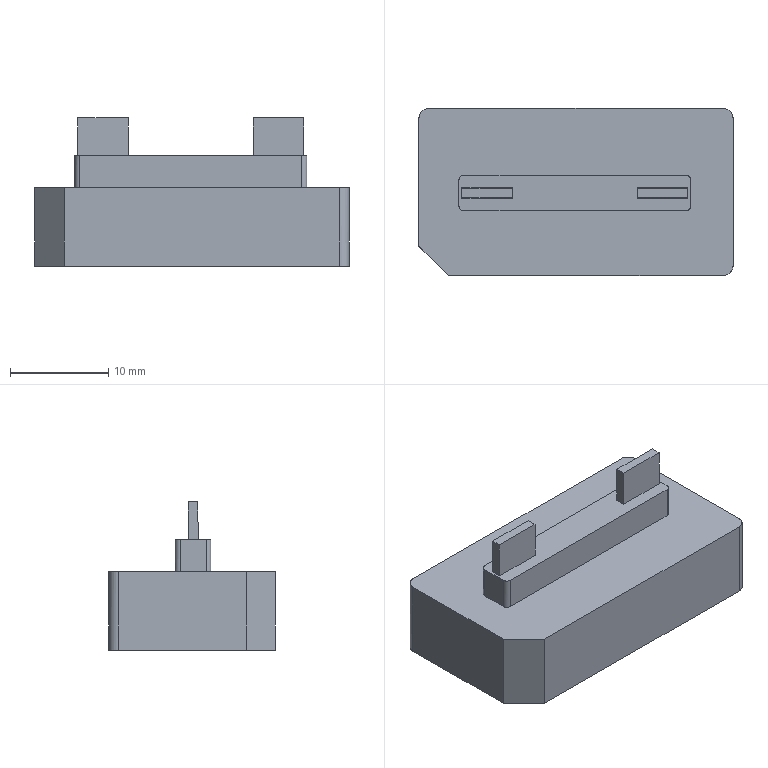NC program | PowerMill | posted by the shop | part box 32 x 17 x 15.109 mm
Lines 1 to 1597 of 56729:
%
G40 G49 G17 G80
( TOOL ID   D10C_1_1 )
( TOOL DIA. 10. TIP RAD 0 LENGTH 70.56 )
( Z = -.071 )
T1 M6
T3
G91 G28 Z0
G0 G90 G54
M08
S8000 M3
G0 X0 Y0 M8
G43 Z10.2 H1
X23.78 Y11.28
Z1.129
G1 Z-.071 F6000
X18.78 F10000
X-18.78
Y5.64
X18.78
Y0
X-18.78
Y-5.64
X18.78
Y-11.28
X-18.78
X-23.78
G0 Z10.2
X-.12 Y0
Z9.879
X24.737 Y5.134
Z.697
G1 Z-.503 F6000
X24.209 F10000
G3 X19.462 Y.387 I0 J-4.748
G1 Y-10.28
G2 X18.462 Y-11.28 I-1. J0
G1 X-18.702
G2 X-19.702 Y-10.28 I0 J1.
G1 Y10.28
G2 X-18.702 Y11.28 I1. J0
G1 X18.462
G2 X19.462 Y10.28 I0 J-1.
G1 Y.387
X16.663
Y-.387
X16.632 Y-1.16
X16.488 Y-1.934
X16.222 Y-2.707
X15.804 Y-3.48
X15.349 Y-4.081
X15.187 Y-4.254
X14.575 Y-4.799
X14.254 Y-5.027
X13.802 Y-5.289
X13.028 Y-5.611
X12.272 Y-5.801
X11.481 Y-5.872
X6.067 Y-5.87
X5.365 Y-5.801
X4.521 Y-5.583
X3.747 Y-5.243
X3.384 Y-5.027
X2.974 Y-4.733
X2.446 Y-4.254
X2.2 Y-3.978
X1.831 Y-3.48
X1.427 Y-2.736
X1.147 Y-1.934
X1.005 Y-1.16
X.979 Y.387
X-1.214
Y-.387
X-1.244 Y-1.16
X-1.389 Y-1.934
X-1.654 Y-2.707
X-2.071 Y-3.48
X-2.44 Y-3.978
X-2.686 Y-4.254
X-3.214 Y-4.733
X-3.623 Y-5.027
X-3.987 Y-5.243
X-4.761 Y-5.583
X-5.605 Y-5.801
X-6.307 Y-5.87
X-11.721 Y-5.872
X-12.495 Y-5.803
X-13.268 Y-5.611
X-14.042 Y-5.289
X-14.493 Y-5.027
X-14.815 Y-4.799
X-15.43 Y-4.254
X-15.589 Y-4.081
X-16.045 Y-3.48
X-16.462 Y-2.707
X-16.73 Y-1.934
X-16.872 Y-1.16
X-16.903 Y-.387
Y.387
X-16.838 Y1.16
X-16.661 Y1.934
X-16.362 Y2.699
X-15.886 Y3.48
X-15.589 Y3.855
X-15.201 Y4.254
X-14.815 Y4.574
X-14.113 Y5.027
X-13.268 Y5.386
X-12.495 Y5.578
X-11.721 Y5.651
X-6.307 Y5.649
X-5.534 Y5.564
X-4.761 Y5.359
X-4.003 Y5.027
X-3.214 Y4.509
X-2.916 Y4.254
X-2.44 Y3.755
X-2.227 Y3.48
X-1.758 Y2.707
X-1.453 Y1.934
X-1.273 Y1.16
X-1.214 Y.387
X.979
X1.036 Y1.16
X1.212 Y1.934
X1.518 Y2.707
X1.987 Y3.48
X2.2 Y3.755
X2.675 Y4.254
X2.974 Y4.509
X3.747 Y5.019
X4.521 Y5.359
X5.294 Y5.564
X6.067 Y5.649
X11.481 Y5.651
X12.255 Y5.578
X13.028 Y5.386
X13.802 Y5.065
X14.575 Y4.574
X14.962 Y4.254
X15.349 Y3.855
X15.651 Y3.48
X16.118 Y2.707
X16.421 Y1.934
X16.602 Y1.16
X16.663 Y.387
X19.462
G0 Z3.315
G1 X24.737 Y5.134
G0 Z.315
G1 Z-.885 F6000
X24.209 F10000
G3 X19.462 Y.387 I0 J-4.748
G1 Y.333
X16.663 Y.387
X16.662 Y.384
X16.663 Y-.387
X16.633 Y-1.137
Y-1.16
X16.49 Y-1.934
X16.224 Y-2.707
X15.807 Y-3.48
X15.349 Y-4.085
X15.193 Y-4.254
X14.575 Y-4.805
X14.259 Y-5.027
X13.802 Y-5.293
X13.028 Y-5.616
X12.29 Y-5.801
X11.481 Y-5.879
X6.067 Y-5.876
X5.343 Y-5.801
X4.521 Y-5.588
X3.747 Y-5.248
X3.374 Y-5.027
X2.974 Y-4.74
X2.44 Y-4.254
X2.2 Y-3.987
X1.826 Y-3.48
X1.427 Y-2.746
X1.142 Y-1.934
X1. Y-1.16
X.971 Y.345
X-1.211 Y.387
X-1.214 Y.211
Y-.387
X-1.237 Y-.971
X-1.24 Y-1.16
X-1.382 Y-1.934
X-1.649 Y-2.707
X-2.066 Y-3.48
X-2.44 Y-3.987
X-2.68 Y-4.254
X-3.214 Y-4.74
X-3.614 Y-5.027
X-3.987 Y-5.248
X-4.761 Y-5.588
X-5.583 Y-5.801
X-6.307 Y-5.876
X-11.721 Y-5.879
X-12.495 Y-5.807
X-13.268 Y-5.616
X-14.042 Y-5.293
X-14.499 Y-5.027
X-14.815 Y-4.805
X-15.434 Y-4.254
X-15.589 Y-4.085
X-16.047 Y-3.48
X-16.464 Y-2.707
X-16.731 Y-1.934
X-16.873 Y-1.16
X-16.874 Y-1.12
X-16.902 Y-.387
Y.384
X-16.903 Y.387
X-16.844 Y1.16
X-16.666 Y1.934
X-16.362 Y2.703
X-15.893 Y3.48
X-15.589 Y3.86
X-15.205 Y4.254
X-14.815 Y4.581
X-14.12 Y5.027
X-13.268 Y5.391
X-12.495 Y5.583
X-11.721 Y5.654
X-6.307 Y5.652
X-5.534 Y5.568
X-4.761 Y5.364
X-3.993 Y5.027
X-3.214 Y4.515
X-2.908 Y4.254
X-2.44 Y3.762
X-2.22 Y3.48
X-1.753 Y2.707
X-1.446 Y1.934
X-1.269 Y1.16
X-1.211 Y.387
X.971 Y.345
Y.387
X1.03 Y1.16
X1.206 Y1.934
X1.513 Y2.707
X1.98 Y3.48
X2.2 Y3.762
X2.668 Y4.254
X2.974 Y4.515
X3.747 Y5.024
X4.521 Y5.364
X5.294 Y5.568
X6.067 Y5.652
X11.481 Y5.654
X12.255 Y5.583
X13.028 Y5.391
X13.802 Y5.069
X14.575 Y4.581
X14.965 Y4.254
X15.349 Y3.86
X15.653 Y3.48
X16.12 Y2.707
X16.426 Y1.934
X16.604 Y1.16
X16.663 Y.387
X19.462 Y.333
Y-10.28
G2 X18.462 Y-11.28 I-1. J0
G1 X-18.702
G2 X-19.702 Y-10.28 I0 J1.
G1 Y10.28
G2 X-18.702 Y11.28 I1. J0
G1 X18.462
G2 X19.462 Y10.28 I0 J-1.
G1 Y.387
G0 Z2.934
G1 X24.737 Y5.134
G0 Z-.066
G1 Z-1.266 F6000
X24.209 F10000
G3 X19.462 Y.387 I0 J-4.748
G1 Y.333
X16.663 Y.387
X16.662 Y.38
Y-.387
X16.634 Y-1.117
X16.633 Y-1.16
X16.492 Y-1.934
X16.225 Y-2.707
X15.81 Y-3.48
X15.349 Y-4.088
X15.197 Y-4.254
X14.575 Y-4.808
X14.264 Y-5.027
X13.802 Y-5.296
X13.028 Y-5.62
X12.309 Y-5.801
X11.481 Y-5.882
X6.067 Y-5.88
X5.321 Y-5.801
X4.521 Y-5.592
X3.747 Y-5.253
X3.366 Y-5.027
X2.974 Y-4.745
X2.433 Y-4.254
X2.2 Y-3.994
X1.82 Y-3.48
X1.427 Y-2.757
X1.138 Y-1.934
X.997 Y-1.16
X.968 Y.345
X-1.207 Y.387
X-1.214 Y.032
Y-.387
X-1.23 Y-.786
X-1.237 Y-1.16
X-1.378 Y-1.934
X-1.645 Y-2.707
X-2.06 Y-3.48
X-2.44 Y-3.994
X-2.673 Y-4.254
X-3.214 Y-4.745
X-3.606 Y-5.027
X-3.987 Y-5.253
X-4.761 Y-5.592
X-5.561 Y-5.801
X-6.307 Y-5.88
X-11.721 Y-5.882
X-12.495 Y-5.81
X-13.268 Y-5.62
X-14.042 Y-5.296
X-14.504 Y-5.027
X-14.815 Y-4.808
X-15.437 Y-4.254
X-15.589 Y-4.088
X-16.05 Y-3.48
X-16.465 Y-2.707
X-16.732 Y-1.934
X-16.873 Y-1.16
X-16.874 Y-1.101
X-16.902 Y-.387
Y.38
X-16.903 Y.387
X-16.844 Y1.16
X-16.668 Y1.934
X-16.362 Y2.706
X-15.895 Y3.48
X-15.589 Y3.864
X-15.209 Y4.254
X-14.815 Y4.584
X-14.126 Y5.027
X-13.268 Y5.396
X-12.495 Y5.586
X-11.721 Y5.658
X-6.307 Y5.656
X-5.534 Y5.572
X-4.761 Y5.368
X-3.987 Y5.029
X-3.214 Y4.521
X-2.901 Y4.254
X-2.44 Y3.77
X-2.214 Y3.48
X-1.748 Y2.707
X-1.441 Y1.934
X-1.265 Y1.16
X-1.207 Y.387
X.968 Y.345
X.967 Y.387
X1.025 Y1.16
X1.201 Y1.934
X1.508 Y2.707
X1.974 Y3.48
X2.2 Y3.77
X2.661 Y4.254
X2.974 Y4.521
X3.744 Y5.027
X4.521 Y5.368
X5.294 Y5.572
X6.067 Y5.656
X11.481 Y5.658
X12.255 Y5.586
X13.028 Y5.396
X13.802 Y5.072
X14.575 Y4.584
X14.969 Y4.254
X15.349 Y3.864
X15.655 Y3.48
X16.121 Y2.707
X16.428 Y1.934
X16.604 Y1.16
X16.663 Y.387
X19.462 Y.333
Y-10.28
G2 X18.462 Y-11.28 I-1. J0
G1 X-18.702
G2 X-19.702 Y-10.28 I0 J1.
G1 Y10.28
G2 X-18.702 Y11.28 I1. J0
G1 X18.462
G2 X19.462 Y10.28 I0 J-1.
G1 Y.387
G0 Z2.552
G1 X24.737 Y5.134
G0 Z-.448
G1 Z-1.648 F6000
X24.209 F10000
G3 X19.462 Y.387 I0 J-4.748
G1 Y.334
X16.663 Y.387
X16.662 Y.377
Y-.387
X16.635 Y-1.098
X16.633 Y-1.16
X16.493 Y-1.934
X16.227 Y-2.707
X15.812 Y-3.48
X15.349 Y-4.092
X15.2 Y-4.254
X14.575 Y-4.812
X14.269 Y-5.027
X13.802 Y-5.299
X13.028 Y-5.623
X12.328 Y-5.801
X11.481 Y-5.885
X6.067 Y-5.883
X5.298 Y-5.801
X4.521 Y-5.597
X3.747 Y-5.258
X3.358 Y-5.027
X2.974 Y-4.751
X2.427 Y-4.254
X2.2 Y-4.001
X1.815 Y-3.48
X1.427 Y-2.768
X1.134 Y-1.934
X.993 Y-1.16
X.965 Y.346
X-1.204 Y.387
X-1.214 Y-.152
Y-.387
X-1.223 Y-.606
X-1.233 Y-1.16
X-1.374 Y-1.934
X-1.64 Y-2.707
X-2.055 Y-3.48
X-2.44 Y-4.001
X-2.667 Y-4.254
X-3.214 Y-4.751
X-3.598 Y-5.027
X-3.987 Y-5.258
X-4.761 Y-5.597
X-5.538 Y-5.801
X-6.307 Y-5.883
X-11.721 Y-5.885
X-12.495 Y-5.814
X-13.268 Y-5.623
X-14.042 Y-5.299
X-14.509 Y-5.027
X-14.815 Y-4.812
X-15.44 Y-4.254
X-15.589 Y-4.092
X-16.052 Y-3.48
X-16.467 Y-2.707
X-16.733 Y-1.934
X-16.873 Y-1.16
X-16.875 Y-1.082
X-16.902 Y-.387
Y.377
X-16.903 Y.387
X-16.845 Y1.16
X-16.669 Y1.934
X-16.363 Y2.707
X-15.898 Y3.48
X-15.589 Y3.868
X-15.212 Y4.254
X-14.815 Y4.587
X-14.132 Y5.027
X-13.268 Y5.399
X-12.495 Y5.589
X-11.721 Y5.661
X-6.307 Y5.659
X-5.534 Y5.576
X-4.761 Y5.373
X-3.987 Y5.034
X-3.214 Y4.527
X-2.894 Y4.254
X-2.44 Y3.777
X-2.209 Y3.48
X-1.743 Y2.707
X-1.437 Y1.934
X-1.262 Y1.16
X-1.204 Y.387
X.965 Y.346
X.964 Y.387
X1.022 Y1.16
X1.197 Y1.934
X1.503 Y2.707
X1.969 Y3.48
X2.2 Y3.777
X2.654 Y4.254
X2.974 Y4.527
X3.734 Y5.027
X4.521 Y5.373
X5.294 Y5.576
X6.067 Y5.659
X11.481 Y5.661
X12.255 Y5.589
X13.028 Y5.399
X13.802 Y5.075
X14.575 Y4.587
X14.972 Y4.254
X15.349 Y3.868
X15.658 Y3.48
X16.122 Y2.709
X16.429 Y1.934
X16.605 Y1.16
X16.663 Y.387
X19.462 Y.334
Y-10.28
G2 X18.462 Y-11.28 I-1. J0
G1 X-18.702
G2 X-19.702 Y-10.28 I0 J1.
G1 Y10.28
G2 X-18.702 Y11.28 I1. J0
G1 X18.462
G2 X19.462 Y10.28 I0 J-1.
G1 Y.387
G0 Z2.17
G1 X24.737 Y5.134
G0 Z-.83
G1 Z-2.03 F6000
X24.209 F10000
G3 X19.462 Y.387 I0 J-4.748
G1 Y.335
X16.663 Y.387
X16.662 Y.374
Y-.387
X16.635 Y-1.079
X16.634 Y-1.16
X16.494 Y-1.934
X16.228 Y-2.707
X15.814 Y-3.48
X15.349 Y-4.095
X15.203 Y-4.254
X14.575 Y-4.815
X14.274 Y-5.027
X13.802 Y-5.303
X13.028 Y-5.626
X12.346 Y-5.801
X11.481 Y-5.889
X6.067 Y-5.887
X5.294 Y-5.804
X4.521 Y-5.601
X3.747 Y-5.264
X3.349 Y-5.027
X2.974 Y-4.757
X2.42 Y-4.254
X2.2 Y-4.009
X1.809 Y-3.48
X1.427 Y-2.778
X1.129 Y-1.934
X.989 Y-1.16
X.961 Y.346
X-1.201 Y.387
X-1.214 Y-.34
Y-.387
X-1.216 Y-.429
X-1.229 Y-1.16
X-1.369 Y-1.934
X-1.635 Y-2.707
X-2.049 Y-3.48
X-2.44 Y-4.009
X-2.66 Y-4.254
X-3.214 Y-4.757
X-3.589 Y-5.027
X-3.987 Y-5.264
X-4.761 Y-5.601
X-5.517 Y-5.801
X-6.307 Y-5.887
X-11.721 Y-5.889
X-12.495 Y-5.817
X-13.268 Y-5.626
X-14.042 Y-5.303
X-14.514 Y-5.027
X-14.815 Y-4.815
X-15.443 Y-4.254
X-15.589 Y-4.095
X-16.054 Y-3.48
X-16.468 Y-2.707
X-16.734 Y-1.934
X-16.874 Y-1.16
X-16.876 Y-1.064
X-16.902 Y-.387
Y.374
X-16.903 Y.387
X-16.845 Y1.16
X-16.67 Y1.934
X-16.365 Y2.707
X-15.9 Y3.48
X-15.589 Y3.871
X-15.216 Y4.254
X-14.815 Y4.591
X-14.139 Y5.027
X-13.268 Y5.402
X-12.495 Y5.593
X-11.721 Y5.664
X-6.307 Y5.662
X-5.534 Y5.58
X-4.761 Y5.377
X-3.987 Y5.039
X-3.214 Y4.533
X-2.887 Y4.254
X-2.44 Y3.784
X-2.203 Y3.48
X-1.738 Y2.707
X-1.433 Y1.934
X-1.258 Y1.16
X-1.201 Y.387
X.961 Y.346
Y.387
X1.018 Y1.16
X1.193 Y1.934
X1.427 Y2.554
X1.478 Y2.643
X1.503 Y2.707
X1.815 Y3.225
X1.963 Y3.48
X2.2 Y3.784
X2.647 Y4.254
X2.974 Y4.533
X3.725 Y5.027
X4.521 Y5.377
X5.294 Y5.58
X6.067 Y5.662
X11.481 Y5.664
X12.255 Y5.593
X13.028 Y5.402
X13.802 Y5.079
X14.575 Y4.591
X14.976 Y4.254
X15.349 Y3.871
X15.66 Y3.48
X16.122 Y2.713
X16.43 Y1.934
X16.605 Y1.16
X16.663 Y.387
X19.462 Y.335
Y-10.28
G2 X18.462 Y-11.28 I-1. J0
G1 X-18.702
G2 X-19.702 Y-10.28 I0 J1.
G1 Y10.28
G2 X-18.702 Y11.28 I1. J0
G1 X18.462
G2 X19.462 Y10.28 I0 J-1.
G1 Y.387
G0 Z1.788
G1 X24.737 Y5.134
G0 Z-1.212
G1 Z-2.412 F6000
X24.209 F10000
G3 X19.462 Y.387 I0 J-4.748
G1 Y.335
X16.663 Y.387
X16.662 Y.371
Y-.387
X16.636 Y-1.06
X16.634 Y-1.16
X16.495 Y-1.934
X16.23 Y-2.707
X16.122 Y-2.94
X15.816 Y-3.48
X15.349 Y-4.098
X15.206 Y-4.254
X14.575 Y-4.818
X14.279 Y-5.027
X13.802 Y-5.306
X13.028 Y-5.63
X12.364 Y-5.801
X11.481 Y-5.892
X6.067 Y-5.89
X5.294 Y-5.808
X4.521 Y-5.606
X3.747 Y-5.269
X3.341 Y-5.027
X2.974 Y-4.763
X2.414 Y-4.254
X2.2 Y-4.016
X1.804 Y-3.48
X1.427 Y-2.789
X1.125 Y-1.934
X.986 Y-1.16
X.958 Y.347
X-1.197 Y.387
X-1.226 Y-1.16
X-1.365 Y-1.934
X-1.63 Y-2.707
X-2.044 Y-3.48
X-2.44 Y-4.016
X-2.654 Y-4.254
X-3.214 Y-4.763
X-3.581 Y-5.027
X-3.987 Y-5.269
X-4.761 Y-5.606
X-5.497 Y-5.801
X-6.307 Y-5.89
X-11.721 Y-5.892
X-12.495 Y-5.82
X-13.268 Y-5.63
X-14.042 Y-5.306
X-14.519 Y-5.027
X-14.815 Y-4.818
X-15.446 Y-4.254
X-15.589 Y-4.098
X-16.056 Y-3.48
X-16.362 Y-2.94
X-16.47 Y-2.707
X-16.735 Y-1.934
X-16.874 Y-1.16
X-16.876 Y-1.046
X-16.902 Y-.387
Y.371
X-16.903 Y.387
X-16.846 Y1.16
X-16.672 Y1.934
X-16.366 Y2.707
X-15.903 Y3.48
X-15.589 Y3.874
X-15.22 Y4.254
X-14.815 Y4.594
X-14.145 Y5.027
X-13.268 Y5.406
X-12.495 Y5.596
X-11.721 Y5.668
X-6.307 Y5.666
X-5.534 Y5.584
X-4.761 Y5.382
X-3.987 Y5.045
X-3.214 Y4.539
X-2.88 Y4.254
X-2.44 Y3.792
X-2.197 Y3.48
X-1.734 Y2.707
X-1.428 Y1.934
X-1.254 Y1.16
X-1.197 Y.387
X.958 Y.347
X.957 Y.387
X1.014 Y1.16
X1.188 Y1.934
X1.427 Y2.565
X1.491 Y2.676
X1.504 Y2.707
X1.655 Y2.958
X1.957 Y3.48
X2.2 Y3.792
X2.64 Y4.254
X2.974 Y4.539
X3.715 Y5.027
X4.521 Y5.382
X5.294 Y5.584
X6.067 Y5.666
X11.481 Y5.668
X12.255 Y5.596
X13.028 Y5.406
X13.802 Y5.082
X14.575 Y4.594
X14.98 Y4.254
X15.349 Y3.874
X15.663 Y3.48
X16.122 Y2.716
X16.432 Y1.934
X16.606 Y1.16
X16.663 Y.387
X19.462 Y.335
Y-10.28
G2 X18.462 Y-11.28 I-1. J0
G1 X-18.702
G2 X-19.702 Y-10.28 I0 J1.
G1 Y10.28
G2 X-18.702 Y11.28 I1. J0
G1 X18.462
G2 X19.462 Y10.28 I0 J-1.
G1 Y.387
G0 Z1.407
G1 X24.737 Y5.134
G0 Z-1.593
G1 Z-2.793 F6000
X24.209 F10000
G3 X19.462 Y.387 I0 J-4.748
G1 Y-10.28
G2 X18.462 Y-11.28 I-1. J0
G1 X-18.702
G2 X-19.702 Y-10.28 I0 J1.
G1 Y10.28
G2 X-18.702 Y11.28 I1. J0
G1 X18.462
G2 X19.462 Y10.28 I0 J-1.
G1 Y.882
X16.642 Y.677
X16.663 Y.387
X16.662 Y.367
Y-.387
X16.637 Y-1.043
X16.634 Y-1.16
X16.496 Y-1.934
X16.231 Y-2.707
X16.122 Y-2.944
X15.818 Y-3.48
X15.349 Y-4.102
X15.209 Y-4.254
X14.575 Y-4.822
X14.284 Y-5.027
X13.802 Y-5.309
X13.028 Y-5.633
X12.381 Y-5.801
X11.481 Y-5.895
X6.067 Y-5.893
X5.294 Y-5.812
X4.521 Y-5.61
X3.747 Y-5.274
X3.332 Y-5.027
X2.974 Y-4.769
X2.407 Y-4.254
X2.2 Y-4.023
X1.798 Y-3.48
X1.427 Y-2.8
X1.121 Y-1.934
X.982 Y-1.16
X.955 Y.348
X-1.194 Y.387
X-1.222 Y-1.16
X-1.361 Y-1.934
X-1.626 Y-2.707
X-2.038 Y-3.48
X-2.44 Y-4.023
X-2.647 Y-4.254
X-3.214 Y-4.769
X-3.572 Y-5.027
X-3.987 Y-5.274
X-4.761 Y-5.61
X-5.476 Y-5.801
X-6.307 Y-5.893
X-11.721 Y-5.895
X-12.495 Y-5.824
X-13.268 Y-5.633
X-14.042 Y-5.309
X-14.524 Y-5.027
X-14.815 Y-4.822
X-15.449 Y-4.254
X-15.589 Y-4.102
X-16.058 Y-3.48
X-16.362 Y-2.944
X-16.471 Y-2.707
X-16.736 Y-1.934
X-16.874 Y-1.16
X-16.877 Y-1.029
X-16.902 Y-.387
Y.367
X-16.903 Y.387
X-16.846 Y1.16
X-16.673 Y1.934
X-16.368 Y2.707
X-15.905 Y3.48
X-15.589 Y3.878
X-15.223 Y4.254
X-14.815 Y4.597
X-14.151 Y5.027
X-13.268 Y5.409
X-12.495 Y5.599
X-11.721 Y5.671
X-6.307 Y5.669
X-5.534 Y5.588
X-4.761 Y5.386
X-3.987 Y5.05
X-3.214 Y4.545
X-2.873 Y4.254
X-2.44 Y3.799
X-2.191 Y3.48
X-1.729 Y2.707
X-1.424 Y1.934
X-1.25 Y1.16
X-1.194 Y.387
X.955 Y.348
X.954 Y.387
X1.01 Y1.16
X1.184 Y1.934
X1.427 Y2.576
X1.951 Y3.48
X2.2 Y3.799
X2.633 Y4.254
X2.974 Y4.545
X3.706 Y5.027
X4.521 Y5.386
X5.294 Y5.588
X6.067 Y5.669
X11.481 Y5.671
X12.255 Y5.599
X13.028 Y5.409
X13.802 Y5.085
X14.575 Y4.597
X14.983 Y4.254
X15.349 Y3.878
X15.665 Y3.48
X16.122 Y2.719
X16.433 Y1.934
X16.606 Y1.16
X16.642 Y.677
X19.462 Y.882
Y.387
G0 Z1.025
G1 X24.737 Y5.134
G0 Z-1.975
G1 Z-3.175 F6000
X24.209 F10000
G3 X19.462 Y.387 I0 J-4.748
G1 Y-10.28
G2 X18.462 Y-11.28 I-1. J0
G1 X-18.702
G2 X-19.702 Y-10.28 I0 J1.
G1 Y10.28
G2 X-18.702 Y11.28 I1. J0
G1 X18.462
G2 X19.462 Y10.28 I0 J-1.
G1 Y.88
X16.642 Y.677
X16.663 Y.387
X16.662 Y.364
Y-.387
X16.637 Y-1.025
X16.635 Y-1.16
X16.496 Y-1.934
X16.232 Y-2.707
X16.122 Y-2.947
X15.82 Y-3.48
X15.762 Y-3.555
X15.348 Y-4.102
X15.232 Y-4.229
X15.213 Y-4.254
X14.575 Y-4.825
X14.289 Y-5.027
X13.802 Y-5.313
X13.028 Y-5.636
X12.398 Y-5.801
X11.481 Y-5.899
X6.067 Y-5.897
X5.294 Y-5.816
X4.521 Y-5.615
X3.747 Y-5.279
X3.324 Y-5.027
X2.974 Y-4.775
X2.401 Y-4.254
X2.2 Y-4.03
X1.793 Y-3.48
X1.427 Y-2.811
X1.117 Y-1.934
X.978 Y-1.16
X.951 Y.348
X-1.191 Y.387
X-1.218 Y-1.16
X-1.357 Y-1.934
X-1.621 Y-2.707
X-2.033 Y-3.48
X-2.44 Y-4.03
X-2.641 Y-4.254
X-3.214 Y-4.775
X-3.564 Y-5.027
X-3.987 Y-5.279
X-4.761 Y-5.615
X-5.456 Y-5.801
X-6.307 Y-5.897
X-11.721 Y-5.899
X-12.495 Y-5.827
X-13.268 Y-5.636
X-14.042 Y-5.313
X-14.529 Y-5.027
X-14.815 Y-4.825
X-15.453 Y-4.254
X-15.472 Y-4.229
X-15.588 Y-4.102
X-16.002 Y-3.555
X-16.06 Y-3.48
X-16.362 Y-2.947
X-16.472 Y-2.707
X-16.736 Y-1.934
X-16.875 Y-1.16
X-16.878 Y-1.012
X-16.902 Y-.387
Y.363
X-16.903 Y.387
X-16.847 Y1.16
X-16.674 Y1.934
X-16.37 Y2.707
X-15.908 Y3.48
X-15.589 Y3.881
X-15.227 Y4.254
X-14.815 Y4.601
X-14.157 Y5.027
X-13.268 Y5.412
X-12.495 Y5.603
X-11.721 Y5.674
X-6.307 Y5.673
X-5.534 Y5.592
X-4.761 Y5.391
X-3.987 Y5.055
X-3.214 Y4.551
X-2.866 Y4.254
X-2.44 Y3.806
X-2.186 Y3.48
X-1.724 Y2.707
X-1.42 Y1.934
X-1.246 Y1.16
X-1.191 Y.387
X.951 Y.348
Y.387
X1.006 Y1.16
X1.18 Y1.934
X1.427 Y2.586
X1.946 Y3.48
X2.2 Y3.806
X2.626 Y4.254
X2.974 Y4.551
X3.696 Y5.027
X4.521 Y5.391
X5.294 Y5.592
X6.067 Y5.673
X11.481 Y5.674
X12.255 Y5.603
X13.028 Y5.412
X13.802 Y5.089
X14.575 Y4.601
X14.987 Y4.254
X15.349 Y3.881
X15.668 Y3.48
X16.122 Y2.723
X16.434 Y1.934
X16.607 Y1.16
X16.642 Y.677
X19.462 Y.88
Y.387
G0 Z.643
G1 X24.737 Y5.134
G0 Z-2.357
G1 Z-3.557 F6000
X24.209 F10000
G3 X19.462 Y.387 I0 J-4.748
G1 Y-10.28
G2 X18.462 Y-11.28 I-1. J0
G1 X-18.702
G2 X-19.702 Y-10.28 I0 J1.
G1 Y10.28
G2 X-18.702 Y11.28 I1. J0
G1 X18.462
G2 X19.462 Y10.28 I0 J-1.
G1 Y.878
X16.642 Y.677
X16.663 Y.387
X16.662 Y.36
Y-.387
X16.638 Y-1.008
X16.635 Y-1.16
X16.497 Y-1.934
X16.234 Y-2.707
X16.122 Y-2.95
X15.822 Y-3.48
X15.701 Y-3.636
X15.348 Y-4.102
X15.255 Y-4.204
X15.216 Y-4.254
X14.575 Y-4.828
X14.294 Y-5.027
X13.802 Y-5.316
X13.028 Y-5.64
X12.415 Y-5.801
X11.481 Y-5.902
X6.067 Y-5.9
X5.294 Y-5.82
X4.521 Y-5.619
X3.747 Y-5.284
X3.316 Y-5.027
X2.974 Y-4.781
X2.394 Y-4.254
X2.2 Y-4.038
X1.787 Y-3.48
X1.427 Y-2.821
X1.113 Y-1.934
X.975 Y-1.16
X.948 Y.349
X-1.187 Y.387
X-1.215 Y-1.16
X-1.353 Y-1.934
X-1.616 Y-2.707
X-2.027 Y-3.48
X-2.44 Y-4.038
X-2.634 Y-4.254
X-3.214 Y-4.781
X-3.556 Y-5.027
X-3.987 Y-5.284
X-4.761 Y-5.619
X-5.435 Y-5.801
X-6.307 Y-5.9
X-11.721 Y-5.902
X-12.495 Y-5.83
X-13.268 Y-5.64
X-14.042 Y-5.316
X-14.534 Y-5.027
X-14.815 Y-4.828
X-15.456 Y-4.254
X-15.495 Y-4.204
X-15.588 Y-4.102
X-15.941 Y-3.636
X-16.062 Y-3.48
X-16.362 Y-2.95
X-16.474 Y-2.707
X-16.737 Y-1.934
X-16.875 Y-1.16
X-16.878 Y-.995
X-16.902 Y-.387
Y.36
X-16.903 Y.387
X-16.847 Y1.16
X-16.675 Y1.934
X-16.371 Y2.707
X-15.91 Y3.48
X-15.589 Y3.884
X-15.23 Y4.254
X-14.815 Y4.604
X-14.163 Y5.027
X-13.268 Y5.416
X-12.495 Y5.606
X-11.721 Y5.678
X-6.307 Y5.676
X-5.534 Y5.595
X-4.761 Y5.395
X-3.987 Y5.06
X-3.214 Y4.557
X-2.86 Y4.254
X-2.44 Y3.814
X-2.18 Y3.48
X-1.719 Y2.707
X-1.415 Y1.934
X-1.243 Y1.16
X-1.187 Y.387
X.948 Y.349
X.947 Y.387
X1.003 Y1.16
X1.175 Y1.934
X1.427 Y2.597
X1.94 Y3.48
X2.2 Y3.814
X2.62 Y4.254
X2.974 Y4.557
X3.687 Y5.027
X4.521 Y5.395
X5.294 Y5.595
X6.067 Y5.676
X11.481 Y5.678
X12.255 Y5.606
X13.028 Y5.416
X13.802 Y5.092
X14.575 Y4.604
X14.99 Y4.254
X15.349 Y3.884
X15.67 Y3.48
X16.122 Y2.726
X16.435 Y1.934
X16.607 Y1.16
X16.642 Y.677
X19.462 Y.878
Y.387
G0 Z.261
G1 X24.737 Y5.134
G0 Z-2.739
G1 Z-3.939 F6000
X24.209 F10000
G3 X19.462 Y.387 I0 J-4.748
G1 Y-10.28
G2 X18.462 Y-11.28 I-1. J0
G1 X-18.702
G2 X-19.702 Y-10.28 I0 J1.
G1 Y10.28
G2 X-18.702 Y11.28 I1. J0
G1 X18.462
G2 X19.462 Y10.28 I0 J-1.
G1 Y.876
X16.642 Y.677
X16.663 Y.387
X16.662 Y.356
Y-.387
X16.638 Y-.992
X16.636 Y-1.16
X16.498 Y-1.934
X16.235 Y-2.707
X16.122 Y-2.954
X15.825 Y-3.48
X15.634 Y-3.724
X15.348 Y-4.102
X15.277 Y-4.18
X15.219 Y-4.254
X14.575 Y-4.832
X14.299 Y-5.027
X13.802 Y-5.319
X13.028 Y-5.643
X12.432 Y-5.801
X11.481 Y-5.905
X6.067 Y-5.904
X5.294 Y-5.824
X4.521 Y-5.624
X3.747 Y-5.289
X3.307 Y-5.027
X2.974 Y-4.787
X2.388 Y-4.254
X2.2 Y-4.045
X1.782 Y-3.48
X1.427 Y-2.832
X1.108 Y-1.934
X.971 Y-1.16
X.945 Y.349
X-1.184 Y.387
X-1.211 Y-1.16
X-1.348 Y-1.934
X-1.611 Y-2.707
X-2.022 Y-3.48
X-2.44 Y-4.045
X-2.628 Y-4.254
X-3.214 Y-4.787
X-3.547 Y-5.027
X-3.987 Y-5.289
X-4.761 Y-5.624
X-5.414 Y-5.801
X-6.307 Y-5.904
X-11.721 Y-5.905
X-12.495 Y-5.834
X-13.268 Y-5.643
X-14.042 Y-5.319
X-14.539 Y-5.027
X-14.815 Y-4.832
X-15.459 Y-4.254
X-15.517 Y-4.18
X-15.588 Y-4.102
X-15.874 Y-3.724
X-16.065 Y-3.48
X-16.362 Y-2.954
X-16.475 Y-2.707
X-16.738 Y-1.934
X-16.876 Y-1.16
X-16.879 Y-.978
X-16.902 Y-.387
Y.356
X-16.903 Y.387
X-16.848 Y1.16
X-16.676 Y1.934
X-16.373 Y2.707
X-15.912 Y3.48
X-15.589 Y3.888
X-15.234 Y4.254
X-14.815 Y4.607
X-14.169 Y5.027
X-13.268 Y5.419
X-12.495 Y5.609
X-11.721 Y5.681
X-6.307 Y5.68
X-5.534 Y5.599
X-4.761 Y5.4
X-3.987 Y5.065
X-3.214 Y4.563
X-2.853 Y4.254
X-2.44 Y3.821
X-2.174 Y3.48
X-1.714 Y2.707
X-1.411 Y1.934
X-1.239 Y1.16
X-1.184 Y.387
X.945 Y.349
X.944 Y.387
X.999 Y1.16
X1.171 Y1.934
X1.427 Y2.608
X1.934 Y3.48
X2.2 Y3.821
X2.613 Y4.254
X2.974 Y4.563
X3.677 Y5.027
X4.521 Y5.4
X5.294 Y5.599
X6.067 Y5.68
X11.481 Y5.681
X12.255 Y5.609
X13.028 Y5.419
X13.802 Y5.095
X14.575 Y4.607
X14.994 Y4.254
X15.349 Y3.888
X15.672 Y3.48
X16.122 Y2.729
X16.436 Y1.934
X16.608 Y1.16
X16.642 Y.677
X19.462 Y.876
Y.387
G0 Z-.136
G1 X24.737 Y5.134
G0 Z-3.136
G1 Z-4.336 F6000
X24.209 F10000
G3 X19.462 Y.387 I0 J-4.748
G1 Y-10.28
G2 X18.462 Y-11.28 I-1. J0
G1 X-18.702
G2 X-19.702 Y-10.28 I0 J1.
G1 Y-1.16
X-17.203
Y1.16
X-17.152 Y1.934
X-17.003 Y2.707
X-16.735 Y3.48
X-16.362 Y4.202
X-15.755 Y5.027
X-15.589 Y5.209
X-14.925 Y5.801
X-14.042 Y6.354
X-13.268 Y6.68
X-12.495 Y6.879
X-11.721 Y6.974
X-10.948 Y6.983
X10.708
X11.481 Y6.974
X12.255 Y6.879
X13.028 Y6.68
X13.802 Y6.354
X14.575 Y5.883
X15.349 Y5.209
X15.515 Y5.027
X16.09 Y4.254
X16.495 Y3.48
X16.763 Y2.707
X16.895 Y2.045
X16.963 Y1.16
Y-1.16
X16.938 Y-1.934
X16.817 Y-2.707
X16.585 Y-3.48
X16.22 Y-4.254
X15.703 Y-5.027
X15.349 Y-5.434
X14.959 Y-5.801
X14.575 Y-6.107
X13.809 Y-6.574
X13.028 Y-6.904
X12.255 Y-7.103
X11.481 Y-7.199
X10.708 Y-7.207
X-10.948
X-11.721 Y-7.199
X-12.495 Y-7.103
X-13.268 Y-6.904
X-14.042 Y-6.578
X-14.815 Y-6.107
X-15.199 Y-5.801
X-15.589 Y-5.434
X-15.943 Y-5.027
X-16.362 Y-4.426
X-16.825 Y-3.48
X-17.057 Y-2.707
X-17.178 Y-1.934
X-17.203 Y-1.16
X-19.702
Y10.28
G2 X-18.702 Y11.28 I1. J0
G1 X18.462
G2 X19.462 Y10.28 I0 J-1.
G1 Y.387
G0 Z-.534
G1 X24.737 Y5.134
G0 Z-3.534
G1 Z-4.734 F6000
X24.209 F10000
G3 X19.462 Y.387 I0 J-4.748
G1 Y-10.28
G2 X18.462 Y-11.28 I-1. J0
G1 X-18.702
G2 X-19.702 Y-10.28 I0 J1.
G1 Y-1.16
X-17.203
Y1.16
X-17.152 Y1.934
X-17.003 Y2.707
X-16.735 Y3.48
X-16.362 Y4.202
X-15.755 Y5.027
X-15.589 Y5.209
X-14.925 Y5.801
X-14.042 Y6.354
X-13.268 Y6.68
X-12.495 Y6.879
X-11.721 Y6.974
X-10.948 Y6.983
X10.708
X11.481 Y6.974
X12.255 Y6.879
X13.028 Y6.68
X13.802 Y6.354
X14.575 Y5.883
X15.349 Y5.209
X15.515 Y5.027
X16.09 Y4.254
X16.495 Y3.48
X16.763 Y2.707
X16.895 Y2.045
X16.963 Y1.16
Y-1.16
X16.938 Y-1.934
X16.817 Y-2.707
X16.585 Y-3.48
X16.22 Y-4.254
X15.703 Y-5.027
X15.349 Y-5.434
X14.959 Y-5.801
X14.575 Y-6.107
X13.809 Y-6.574
X13.028 Y-6.904
X12.255 Y-7.103
X11.481 Y-7.199
X10.708 Y-7.207
X-10.948
X-11.721 Y-7.199
X-12.495 Y-7.103
X-13.268 Y-6.904
X-14.042 Y-6.578
X-14.815 Y-6.107
X-15.199 Y-5.801
X-15.589 Y-5.434
X-15.943 Y-5.027
X-16.362 Y-4.426
X-16.825 Y-3.48
X-17.057 Y-2.707
X-17.178 Y-1.934
X-17.203 Y-1.16
X-19.702
Y10.28
G2 X-18.702 Y11.28 I1. J0
G1 X18.462
G2 X19.462 Y10.28 I0 J-1.
G1 Y.387
G0 Z-.932
G1 X24.737 Y5.134
G0 Z-3.932
G1 Z-5.132 F6000
X24.209 F10000
G3 X19.462 Y.387 I0 J-4.748
G1 Y-10.28
G2 X18.462 Y-11.28 I-1. J0
G1 X-18.702
G2 X-19.702 Y-10.28 I0 J1.
G1 Y-1.16
X-17.203
Y1.16
X-17.152 Y1.934
X-17.003 Y2.707
X-16.735 Y3.48
X-16.362 Y4.202
X-15.755 Y5.027
X-15.589 Y5.209
X-14.925 Y5.801
X-14.042 Y6.354
X-13.268 Y6.68
X-12.495 Y6.879
X-11.721 Y6.974
X-10.948 Y6.983
X10.708
X11.481 Y6.974
X12.255 Y6.879
X13.028 Y6.68
X13.802 Y6.354
X14.575 Y5.883
X15.349 Y5.209
X15.515 Y5.027
X16.09 Y4.254
X16.495 Y3.48
X16.763 Y2.707
X16.895 Y2.045
X16.963 Y1.16
Y-1.16
X16.938 Y-1.934
X16.817 Y-2.707
X16.585 Y-3.48
X16.22 Y-4.254
X15.703 Y-5.027
X15.349 Y-5.434
X14.959 Y-5.801
X14.575 Y-6.107
X13.809 Y-6.574
X13.028 Y-6.904
X12.255 Y-7.103
X11.481 Y-7.199
X10.708 Y-7.207
X-10.948
X-11.721 Y-7.199
X-12.495 Y-7.103
X-13.268 Y-6.904
X-14.042 Y-6.578
X-14.815 Y-6.107
X-15.199 Y-5.801
X-15.589 Y-5.434
X-15.943 Y-5.027
X-16.362 Y-4.426
X-16.825 Y-3.48
X-17.057 Y-2.707
X-17.178 Y-1.934
X-17.203 Y-1.16
X-19.702
Y10.28
G2 X-18.702 Y11.28 I1. J0
G1 X18.462
G2 X19.462 Y10.28 I0 J-1.
G1 Y.387
G0 Z-1.329
G1 X24.737 Y5.134
G0 Z-4.329
G1 Z-5.529 F6000
X24.209 F10000
G3 X19.462 Y.387 I0 J-4.748
G1 Y-10.28
G2 X18.462 Y-11.28 I-1. J0
G1 X-18.702
G2 X-19.702 Y-10.28 I0 J1.
G1 Y-1.16
X-17.203
Y1.16
X-17.152 Y1.934
X-17.003 Y2.707
X-16.735 Y3.48
X-16.362 Y4.202
X-15.755 Y5.027
X-15.589 Y5.209
X-14.925 Y5.801
X-14.042 Y6.354
X-13.268 Y6.68
X-12.495 Y6.879
X-11.721 Y6.974
X-10.948 Y6.983
X10.708
X11.481 Y6.974
X12.255 Y6.879
X13.028 Y6.68
X13.802 Y6.354
X14.575 Y5.883
X15.349 Y5.209
X15.515 Y5.027
X16.09 Y4.254
X16.495 Y3.48
X16.763 Y2.707
X16.895 Y2.045
X16.963 Y1.16
Y-1.16
X16.938 Y-1.934
X16.817 Y-2.707
X16.585 Y-3.48
X16.221 Y-4.254
X15.703 Y-5.027
X15.349 Y-5.434
X14.959 Y-5.801
X14.575 Y-6.107
X13.809 Y-6.574
X13.028 Y-6.904
X12.255 Y-7.103
X11.481 Y-7.199
X10.708 Y-7.207
X-10.948
X-11.721 Y-7.199
X-12.495 Y-7.103
X-13.268 Y-6.904
X-14.042 Y-6.578
X-14.815 Y-6.107
X-15.199 Y-5.801
X-15.589 Y-5.434
X-15.943 Y-5.027
X-16.362 Y-4.426
X-16.825 Y-3.48
X-17.057 Y-2.707
X-17.178 Y-1.934
X-17.203 Y-1.16
X-19.702
Y10.28
G2 X-18.702 Y11.28 I1. J0
G1 X18.462
G2 X19.462 Y10.28 I0 J-1.
G1 Y.387
G0 Z-1.727
G1 X24.737 Y5.134
G0 Z-4.727
G1 Z-5.927 F6000
X24.209 F10000
G3 X19.462 Y.387 I0 J-4.748
G1 Y-10.28
G2 X18.462 Y-11.28 I-1. J0
G1 X-18.702
G2 X-19.702 Y-10.28 I0 J1.